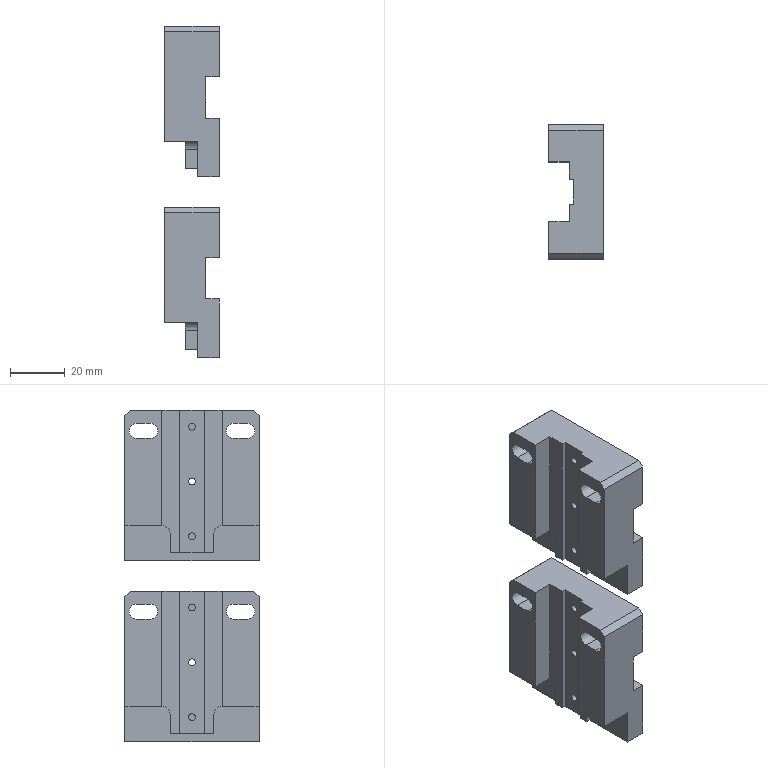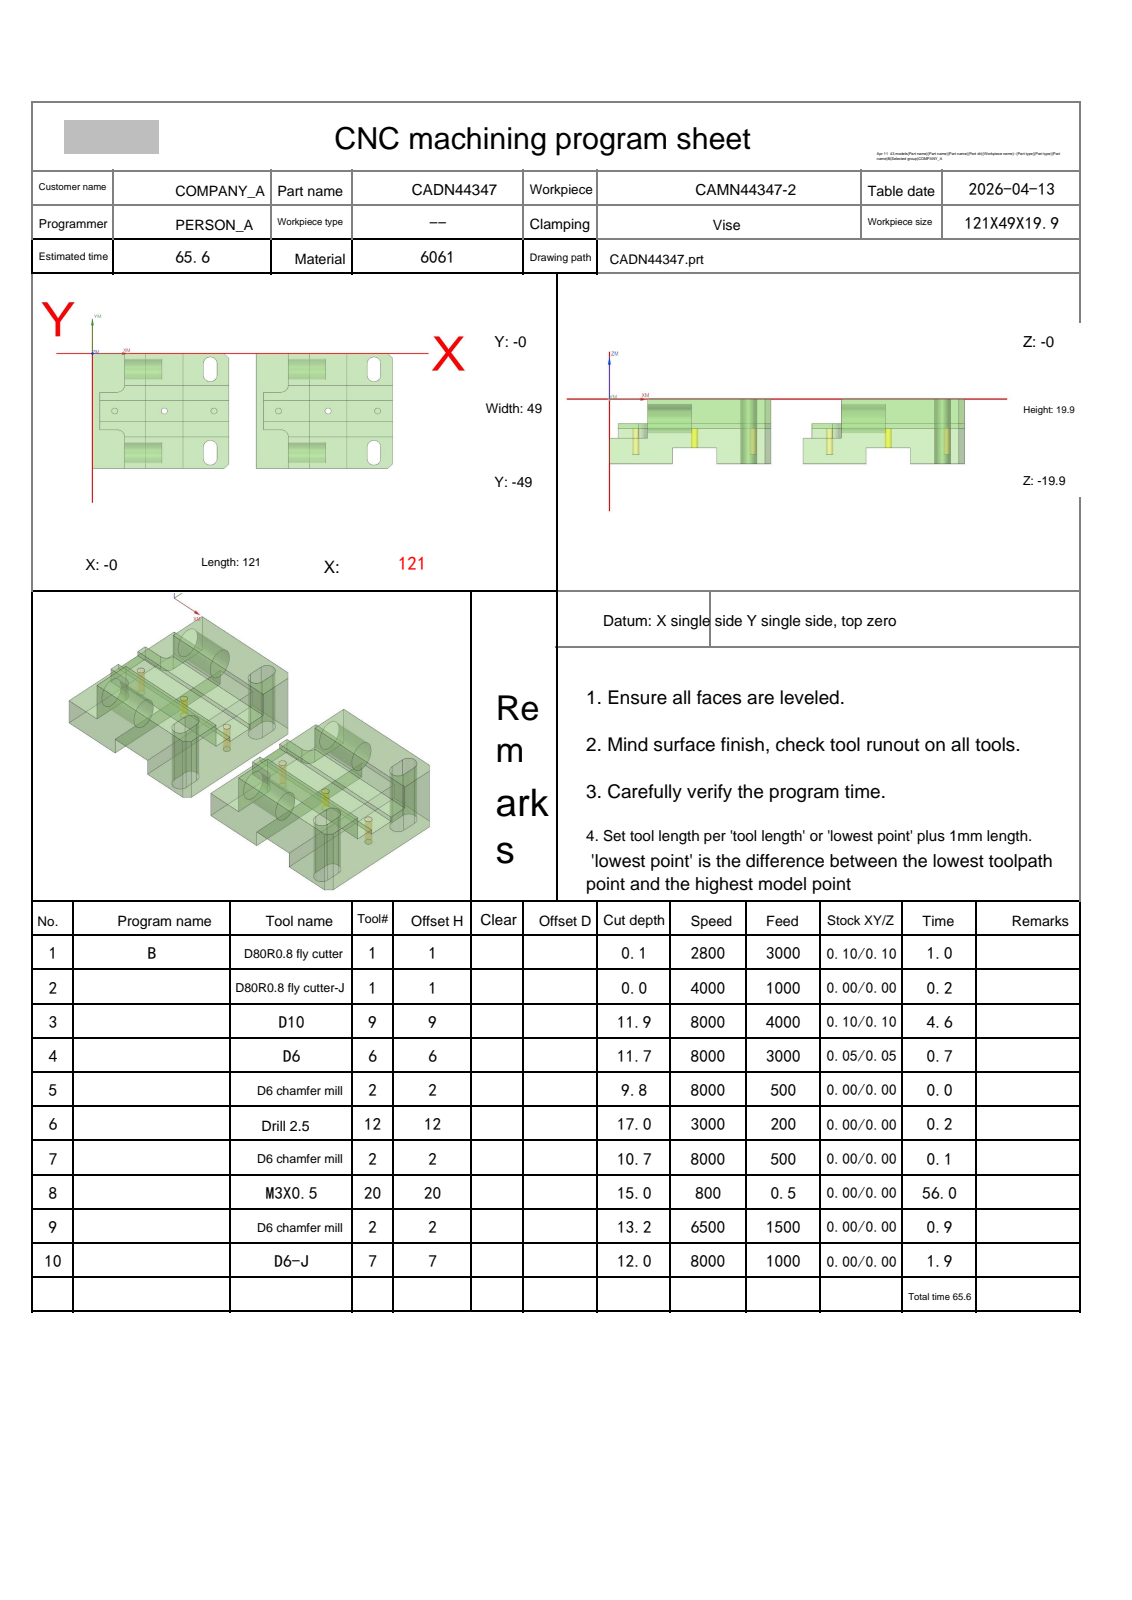NC program | NX | posted by the shop | part box 19.9 x 49 x 121 mm
Lines 1 to 119 of 6263:
%
O0001
(Machine time: 115.43 MIN)
(===Total Tool:7===)
(T1=D80R0.8 fly cutter D=80.  R=0.8  D-  H01 Z=0.    )
(T9=D10     D=10.  R=0.   D-  H09 Z=-11.9 )
(T6=D6      D=6.   R=0.   D-  H06 Z=-11.75)
(T2=D6 chamfer mill   D=6.   R=0.   D-  H02 Z=-13.2 )
(T12=Drill 2.5  D=2.5  DR_a=118 D-  H12 Z=-17.  )
(T20=M3X0.5 D=2.5  DR_a=180 D-  H20 Z=-15.  )
(T7=D6-J    D=6.   R=0.   D7  H07 Z=-12.  )
G80 G90 G17 G49 G40
G91 G28 Z0
M01
N1 T01 M06
(D80R0.8 fly cutter  D=80. R=0.8 H=01 ce=0.10 di=0.10)
G00 G90 G54 X-52.097 Y-24.5 M03 S2800
G43 H01 Z20.
M08
Z6.51
G01 Z4.51 F3000.
X-40.097
X161.097
X173.097
Z6.51
G00 X-52.097
Z6.02
G01 Z4.02
X-40.097
X161.097
X173.097
Z6.02
G00 X-52.097
Z5.53
G01 Z3.53
X-40.097
X161.097
X173.097
Z5.53
G00 X-52.097
Z5.04
G01 Z3.04
X-40.097
X161.097
X173.097
Z5.04
G00 Z20.
X-52.097
Z4.55
G01 Z2.55
X-40.097
X161.097
X173.097
Z4.55
G00 Z20.
X-52.097
Z4.06
G01 Z2.06
X-40.097
X161.097
X173.097
Z4.06
G00 Z20.
X-52.097
Z3.57
G01 Z1.57
X-40.097
X161.097
X173.097
Z3.57
G00 Z20.
X-52.097
Z3.08
G01 Z1.08
X-40.097
X161.097
X173.097
Z3.08
G00 Z20.
X-52.097
Z2.59
G01 Z.59
X-40.097
X161.097
X173.097
Z2.59
G00 Z20.
X-52.097
Z2.1
G01 Z.1
X-40.097
X161.097
X173.097
Z2.1
G00 Z20.
G91 G28 Z0.0
M05
M09
G91 G28 Z0.0
M01
N2 T01 M06
(D80R0.8 fly cutter-J  D=80. R=0.8 H=01 ce=0.00 di=0.00)
G00 G90 G54 X-51.999 Y-24.5 M03 S4000
G43 H01 Z20.
M08
Z2.
G01 Z0.0 F1000.
X-39.999
X160.999
X172.999
Z2.
G00 Z20.
G91 G28 Z0.0
M05
M09
G91 G28 Z0.0
M01